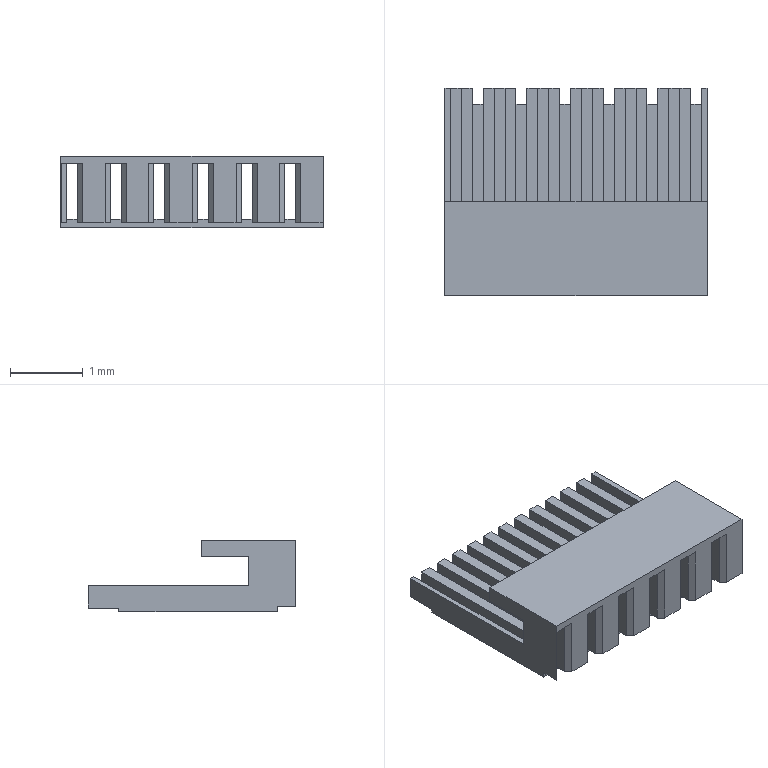Part | Creo | 1 solid | 170 faces | box 3.6 x 2.85 x 0.98 mm | volume 3.689 mm3 | plane 170